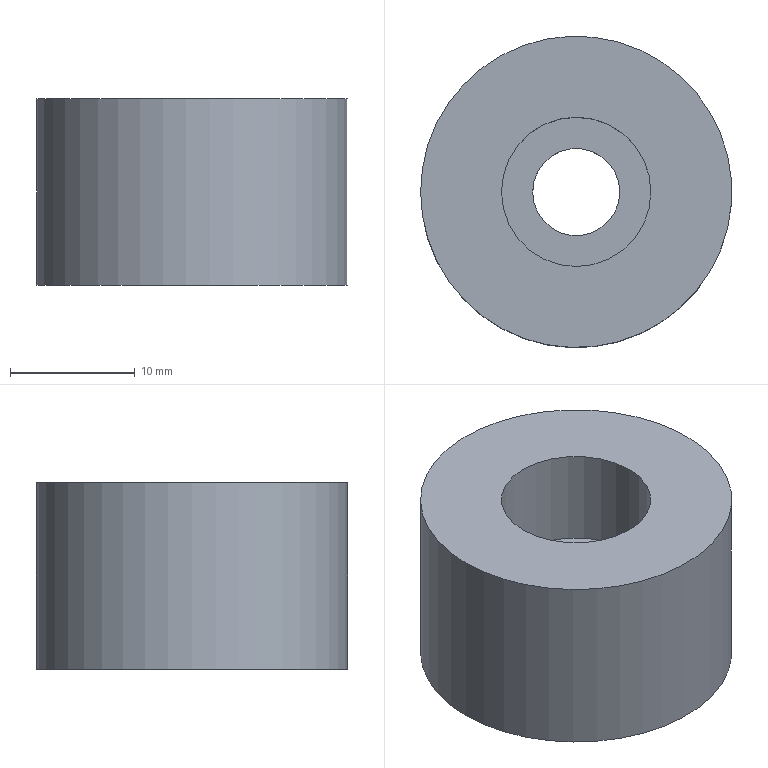Part | NX | features LIN_SOLID_COLOR 2 | 1 solid | 6 faces | box 25 x 25 x 15 mm | volume 6189 mm3 | cylinder 3 | plane 3 | commonest cylinder face diameters 7 x1 12 x1 25 x1
STEP:
#1=CARTESIAN_POINT('',(238.5,113.,-11.5));
#2=VERTEX_POINT('',#1);
#3=CARTESIAN_POINT('',(251.,113.,-11.5));
#4=DIRECTION('',(0.,0.,1.));
#5=DIRECTION('',(-1.,0.,0.));
#6=AXIS2_PLACEMENT_3D('',#3,#4,#5);
#7=CIRCLE('',#6,12.5);
#8=EDGE_CURVE('',#2,#2,#7,.T.);
#9=ORIENTED_EDGE('',*,*,#8,.T.);
#10=EDGE_LOOP('',(#9));
#11=FACE_BOUND('',#10,.T.);
#12=CARTESIAN_POINT('',(238.5,113.,3.5));
#13=VERTEX_POINT('',#12);
#14=CARTESIAN_POINT('',(251.,113.,3.5));
#15=DIRECTION('',(0.,0.,1.));
#16=DIRECTION('',(-1.,0.,0.));
#17=AXIS2_PLACEMENT_3D('',#14,#15,#16);
#18=CIRCLE('',#17,12.5);
#19=EDGE_CURVE('',#13,#13,#18,.F.);
#20=ORIENTED_EDGE('',*,*,#19,.T.);
#21=EDGE_LOOP('',(#20));
#22=FACE_BOUND('',#21,.T.);
#23=CARTESIAN_POINT('',(251.,113.,55.));
#24=DIRECTION('',(0.,0.,1.));
#25=DIRECTION('',(-1.,0.,0.));
#26=AXIS2_PLACEMENT_3D('',#23,#24,#25);
#27=CYLINDRICAL_SURFACE('',#26,12.5);
#28=ADVANCED_FACE('',(#11,#22),#27,.T.);
#29=CARTESIAN_POINT('',(257.,113.,-4.5));
#30=VERTEX_POINT('',#29);
#31=CARTESIAN_POINT('',(251.,113.,-4.5));
#32=DIRECTION('',(0.,0.,1.));
#33=DIRECTION('',(1.,0.,0.));
#34=AXIS2_PLACEMENT_3D('',#31,#32,#33);
#35=CIRCLE('',#34,6.);
#36=EDGE_CURVE('',#30,#30,#35,.T.);
#37=ORIENTED_EDGE('',*,*,#36,.F.);
#38=EDGE_LOOP('',(#37));
#39=FACE_BOUND('',#38,.T.);
#40=CARTESIAN_POINT('',(257.,113.,3.5));
#41=VERTEX_POINT('',#40);
#42=CARTESIAN_POINT('',(251.,113.,3.5));
#43=DIRECTION('',(0.,0.,1.));
#44=DIRECTION('',(1.,0.,0.));
#45=AXIS2_PLACEMENT_3D('',#42,#43,#44);
#46=CIRCLE('',#45,6.);
#47=EDGE_CURVE('',#41,#41,#46,.F.);
#48=ORIENTED_EDGE('',*,*,#47,.F.);
#49=EDGE_LOOP('',(#48));
#50=FACE_BOUND('',#49,.T.);
#51=CARTESIAN_POINT('',(251.,113.,3.5));
#52=DIRECTION('',(0.,0.,1.));
#53=DIRECTION('',(-1.,0.,0.));
#54=AXIS2_PLACEMENT_3D('',#51,#52,#53);
#55=CYLINDRICAL_SURFACE('',#54,6.);
#56=ADVANCED_FACE('',(#39,#50),#55,.F.);
#57=ORIENTED_EDGE('',*,*,#8,.F.);
#58=EDGE_LOOP('',(#57));
#59=FACE_BOUND('',#58,.T.);
#60=CARTESIAN_POINT('',(254.5,113.,-11.5));
#61=VERTEX_POINT('',#60);
#62=CARTESIAN_POINT('',(251.,113.,-11.5));
#63=DIRECTION('',(0.,0.,1.));
#64=DIRECTION('',(1.,0.,0.));
#65=AXIS2_PLACEMENT_3D('',#62,#63,#64);
#66=CIRCLE('',#65,3.5);
#67=EDGE_CURVE('',#61,#61,#66,.F.);
#68=ORIENTED_EDGE('',*,*,#67,.F.);
#69=EDGE_LOOP('',(#68));
#70=FACE_BOUND('',#69,.T.);
#71=CARTESIAN_POINT('',(226.,76.,-11.5));
#72=DIRECTION('',(0.,0.,1.));
#73=DIRECTION('',(-1.,0.,0.));
#74=AXIS2_PLACEMENT_3D('',#71,#72,#73);
#75=PLANE('',#74);
#76=ADVANCED_FACE('',(#59,#70),#75,.F.);
#77=CARTESIAN_POINT('',(254.5,113.,-4.5));
#78=VERTEX_POINT('',#77);
#79=CARTESIAN_POINT('',(251.,113.,-4.5));
#80=DIRECTION('',(0.,0.,1.));
#81=DIRECTION('',(1.,0.,0.));
#82=AXIS2_PLACEMENT_3D('',#79,#80,#81);
#83=CIRCLE('',#82,3.5);
#84=EDGE_CURVE('',#78,#78,#83,.F.);
#85=ORIENTED_EDGE('',*,*,#84,.F.);
#86=EDGE_LOOP('',(#85));
#87=FACE_BOUND('',#86,.T.);
#88=ORIENTED_EDGE('',*,*,#67,.T.);
#89=EDGE_LOOP('',(#88));
#90=FACE_BOUND('',#89,.T.);
#91=CARTESIAN_POINT('',(251.,113.,-21.5));
#92=DIRECTION('',(0.,0.,1.));
#93=DIRECTION('',(-1.,0.,0.));
#94=AXIS2_PLACEMENT_3D('',#91,#92,#93);
#95=CYLINDRICAL_SURFACE('',#94,3.5);
#96=ADVANCED_FACE('',(#87,#90),#95,.F.);
#97=ORIENTED_EDGE('',*,*,#36,.T.);
#98=EDGE_LOOP('',(#97));
#99=FACE_BOUND('',#98,.T.);
#100=ORIENTED_EDGE('',*,*,#84,.T.);
#101=EDGE_LOOP('',(#100));
#102=FACE_BOUND('',#101,.T.);
#103=CARTESIAN_POINT('',(226.,76.,-4.5));
#104=DIRECTION('',(0.,0.,1.));
#105=DIRECTION('',(-1.,0.,0.));
#106=AXIS2_PLACEMENT_3D('',#103,#104,#105);
#107=PLANE('',#106);
#108=ADVANCED_FACE('',(#99,#102),#107,.T.);
#109=ORIENTED_EDGE('',*,*,#19,.F.);
#110=EDGE_LOOP('',(#109));
#111=FACE_BOUND('',#110,.T.);
#112=ORIENTED_EDGE('',*,*,#47,.T.);
#113=EDGE_LOOP('',(#112));
#114=FACE_BOUND('',#113,.T.);
#115=CARTESIAN_POINT('',(251.,113.,3.5));
#116=DIRECTION('',(0.,0.,1.));
#117=DIRECTION('',(-1.,0.,0.));
#118=AXIS2_PLACEMENT_3D('',#115,#116,#117);
#119=PLANE('',#118);
#120=ADVANCED_FACE('',(#111,#114),#119,.T.);
#121=CLOSED_SHELL('',(#28,#56,#76,#96,#108,#120));
#122=MANIFOLD_SOLID_BREP('',#121);
#123=(LENGTH_UNIT()NAMED_UNIT(*)SI_UNIT(.MILLI.,.METRE.));
#124=UNCERTAINTY_MEASURE_WITH_UNIT(LENGTH_MEASURE(0.00001),#123,'','');
#125=(NAMED_UNIT(*)PLANE_ANGLE_UNIT()SI_UNIT($,.RADIAN.));
#126=(NAMED_UNIT(*)SI_UNIT($,.STERADIAN.)SOLID_ANGLE_UNIT());
#127=(GEOMETRIC_REPRESENTATION_CONTEXT(3)GLOBAL_UNCERTAINTY_ASSIGNED_CONTEXT((#124))GLOBAL_UNIT_ASSIGNED_CONTEXT((#123,#125,#126))REPRESENTATION_CONTEXT('',''));
#128=ADVANCED_BREP_SHAPE_REPRESENTATION('',(#122),#127);